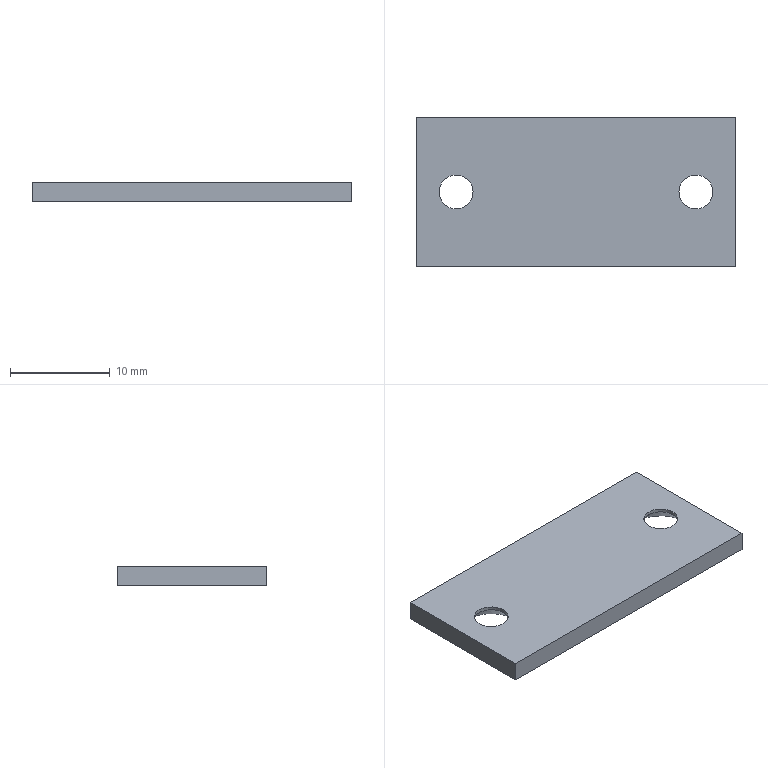Part | SolidWorks | features BaseBody 1 | 1 solid | 14 faces | box 32 x 15 x 2 mm | volume 884.669 mm3 | plane 6 | cone 4 | cylinder 4 | commonest cylinder face diameters 3.4 x4
STEP:
#1=CARTESIAN_POINT('',(-10.3,0.,1.66));
#2=VERTEX_POINT('',#1);
#3=CARTESIAN_POINT('',(-13.7,0.,1.66));
#4=VERTEX_POINT('',#3);
#5=CARTESIAN_POINT('',(-12.,0.,1.66));
#6=DIRECTION('',(0.,0.,-1.));
#7=DIRECTION('',(-1.,0.,0.));
#8=AXIS2_PLACEMENT_3D('',#5,#6,#7);
#9=CIRCLE('',#8,1.7);
#10=EDGE_CURVE('',#2,#4,#9,.T.);
#11=ORIENTED_EDGE('',*,*,#10,.F.);
#12=CARTESIAN_POINT('',(-8.64,0.,0.));
#13=VERTEX_POINT('',#12);
#14=CARTESIAN_POINT('',(-8.64,0.,0.));
#15=DIRECTION('',(0.7071,0.,-0.7071));
#16=VECTOR('',#15,1000.);
#17=LINE('',#14,#16);
#18=EDGE_CURVE('',#2,#13,#17,.T.);
#19=ORIENTED_EDGE('',*,*,#18,.T.);
#20=CARTESIAN_POINT('',(-15.36,0.,0.));
#21=VERTEX_POINT('',#20);
#22=CARTESIAN_POINT('',(-12.,0.,0.));
#23=DIRECTION('',(0.,0.,-1.));
#24=DIRECTION('',(-1.,0.,0.));
#25=AXIS2_PLACEMENT_3D('',#22,#23,#24);
#26=CIRCLE('',#25,3.36);
#27=EDGE_CURVE('',#13,#21,#26,.T.);
#28=ORIENTED_EDGE('',*,*,#27,.T.);
#29=CARTESIAN_POINT('',(-15.36,0.,0.));
#30=DIRECTION('',(-0.7071,0.,-0.7071));
#31=VECTOR('',#30,1000.);
#32=LINE('',#29,#31);
#33=EDGE_CURVE('',#4,#21,#32,.T.);
#34=ORIENTED_EDGE('',*,*,#33,.F.);
#35=EDGE_LOOP('',(#11,#19,#28,#34));
#36=FACE_OUTER_BOUND('',#35,.T.);
#37=CARTESIAN_POINT('',(-12.,0.,0.));
#38=DIRECTION('',(0.,0.,-1.));
#39=DIRECTION('',(-1.,0.,0.));
#40=AXIS2_PLACEMENT_3D('',#37,#38,#39);
#41=CONICAL_SURFACE('',#40,3.36,0.7854);
#42=ADVANCED_FACE('',(#36),#41,.F.);
#43=CARTESIAN_POINT('',(-10.3,0.,2.));
#44=VERTEX_POINT('',#43);
#45=CARTESIAN_POINT('',(-13.7,0.,2.));
#46=VERTEX_POINT('',#45);
#47=CARTESIAN_POINT('',(-12.,0.,2.));
#48=DIRECTION('',(0.,0.,-1.));
#49=DIRECTION('',(-1.,0.,0.));
#50=AXIS2_PLACEMENT_3D('',#47,#48,#49);
#51=CIRCLE('',#50,1.7);
#52=EDGE_CURVE('',#44,#46,#51,.T.);
#53=ORIENTED_EDGE('',*,*,#52,.F.);
#54=CARTESIAN_POINT('',(-10.3,0.,0.));
#55=DIRECTION('',(0.,0.,-1.));
#56=VECTOR('',#55,1000.);
#57=LINE('',#54,#56);
#58=EDGE_CURVE('',#44,#2,#57,.T.);
#59=ORIENTED_EDGE('',*,*,#58,.T.);
#60=ORIENTED_EDGE('',*,*,#10,.T.);
#61=CARTESIAN_POINT('',(-13.7,0.,0.));
#62=DIRECTION('',(0.,0.,-1.));
#63=VECTOR('',#62,1000.);
#64=LINE('',#61,#63);
#65=EDGE_CURVE('',#46,#4,#64,.T.);
#66=ORIENTED_EDGE('',*,*,#65,.F.);
#67=EDGE_LOOP('',(#53,#59,#60,#66));
#68=FACE_OUTER_BOUND('',#67,.T.);
#69=CARTESIAN_POINT('',(-12.,0.,0.));
#70=DIRECTION('',(0.,0.,-1.));
#71=DIRECTION('',(-1.,0.,0.));
#72=AXIS2_PLACEMENT_3D('',#69,#70,#71);
#73=CYLINDRICAL_SURFACE('',#72,1.7);
#74=ADVANCED_FACE('',(#68),#73,.F.);
#75=CARTESIAN_POINT('',(13.7,0.,1.66));
#76=VERTEX_POINT('',#75);
#77=CARTESIAN_POINT('',(10.3,0.,1.66));
#78=VERTEX_POINT('',#77);
#79=CARTESIAN_POINT('',(12.,0.,1.66));
#80=DIRECTION('',(0.,0.,-1.));
#81=DIRECTION('',(-1.,0.,0.));
#82=AXIS2_PLACEMENT_3D('',#79,#80,#81);
#83=CIRCLE('',#82,1.7);
#84=EDGE_CURVE('',#76,#78,#83,.T.);
#85=ORIENTED_EDGE('',*,*,#84,.F.);
#86=CARTESIAN_POINT('',(15.36,0.,0.));
#87=VERTEX_POINT('',#86);
#88=CARTESIAN_POINT('',(15.36,0.,0.));
#89=DIRECTION('',(0.7071,0.,-0.7071));
#90=VECTOR('',#89,1000.);
#91=LINE('',#88,#90);
#92=EDGE_CURVE('',#76,#87,#91,.T.);
#93=ORIENTED_EDGE('',*,*,#92,.T.);
#94=CARTESIAN_POINT('',(8.64,0.,0.));
#95=VERTEX_POINT('',#94);
#96=CARTESIAN_POINT('',(12.,0.,0.));
#97=DIRECTION('',(0.,0.,-1.));
#98=DIRECTION('',(-1.,0.,0.));
#99=AXIS2_PLACEMENT_3D('',#96,#97,#98);
#100=CIRCLE('',#99,3.36);
#101=EDGE_CURVE('',#87,#95,#100,.T.);
#102=ORIENTED_EDGE('',*,*,#101,.T.);
#103=CARTESIAN_POINT('',(8.64,0.,0.));
#104=DIRECTION('',(-0.7071,0.,-0.7071));
#105=VECTOR('',#104,1000.);
#106=LINE('',#103,#105);
#107=EDGE_CURVE('',#78,#95,#106,.T.);
#108=ORIENTED_EDGE('',*,*,#107,.F.);
#109=EDGE_LOOP('',(#85,#93,#102,#108));
#110=FACE_OUTER_BOUND('',#109,.T.);
#111=CARTESIAN_POINT('',(12.,0.,0.));
#112=DIRECTION('',(0.,0.,-1.));
#113=DIRECTION('',(-1.,0.,0.));
#114=AXIS2_PLACEMENT_3D('',#111,#112,#113);
#115=CONICAL_SURFACE('',#114,3.36,0.7854);
#116=ADVANCED_FACE('',(#110),#115,.F.);
#117=CARTESIAN_POINT('',(13.7,0.,2.));
#118=VERTEX_POINT('',#117);
#119=CARTESIAN_POINT('',(10.3,0.,2.));
#120=VERTEX_POINT('',#119);
#121=CARTESIAN_POINT('',(12.,0.,2.));
#122=DIRECTION('',(0.,0.,-1.));
#123=DIRECTION('',(-1.,0.,0.));
#124=AXIS2_PLACEMENT_3D('',#121,#122,#123);
#125=CIRCLE('',#124,1.7);
#126=EDGE_CURVE('',#118,#120,#125,.T.);
#127=ORIENTED_EDGE('',*,*,#126,.F.);
#128=CARTESIAN_POINT('',(13.7,0.,0.));
#129=DIRECTION('',(0.,0.,-1.));
#130=VECTOR('',#129,1000.);
#131=LINE('',#128,#130);
#132=EDGE_CURVE('',#118,#76,#131,.T.);
#133=ORIENTED_EDGE('',*,*,#132,.T.);
#134=ORIENTED_EDGE('',*,*,#84,.T.);
#135=CARTESIAN_POINT('',(10.3,0.,0.));
#136=DIRECTION('',(0.,0.,-1.));
#137=VECTOR('',#136,1000.);
#138=LINE('',#135,#137);
#139=EDGE_CURVE('',#120,#78,#138,.T.);
#140=ORIENTED_EDGE('',*,*,#139,.F.);
#141=EDGE_LOOP('',(#127,#133,#134,#140));
#142=FACE_OUTER_BOUND('',#141,.T.);
#143=CARTESIAN_POINT('',(12.,0.,0.));
#144=DIRECTION('',(0.,0.,-1.));
#145=DIRECTION('',(-1.,0.,0.));
#146=AXIS2_PLACEMENT_3D('',#143,#144,#145);
#147=CYLINDRICAL_SURFACE('',#146,1.7);
#148=ADVANCED_FACE('',(#142),#147,.F.);
#149=CARTESIAN_POINT('',(12.,0.,0.));
#150=DIRECTION('',(0.,0.,-1.));
#151=DIRECTION('',(-1.,0.,0.));
#152=AXIS2_PLACEMENT_3D('',#149,#150,#151);
#153=CIRCLE('',#152,3.36);
#154=EDGE_CURVE('',#95,#87,#153,.T.);
#155=ORIENTED_EDGE('',*,*,#154,.F.);
#156=ORIENTED_EDGE('',*,*,#101,.F.);
#157=EDGE_LOOP('',(#155,#156));
#158=FACE_BOUND('',#157,.T.);
#159=CARTESIAN_POINT('',(-12.,0.,0.));
#160=DIRECTION('',(0.,0.,-1.));
#161=DIRECTION('',(-1.,0.,0.));
#162=AXIS2_PLACEMENT_3D('',#159,#160,#161);
#163=CIRCLE('',#162,3.36);
#164=EDGE_CURVE('',#21,#13,#163,.T.);
#165=ORIENTED_EDGE('',*,*,#164,.F.);
#166=ORIENTED_EDGE('',*,*,#27,.F.);
#167=EDGE_LOOP('',(#165,#166));
#168=FACE_BOUND('',#167,.T.);
#169=CARTESIAN_POINT('',(16.,-7.5,0.));
#170=VERTEX_POINT('',#169);
#171=CARTESIAN_POINT('',(16.,7.5,0.));
#172=VERTEX_POINT('',#171);
#173=CARTESIAN_POINT('',(16.,-7.5,0.));
#174=DIRECTION('',(0.,1.,0.));
#175=VECTOR('',#174,1000.);
#176=LINE('',#173,#175);
#177=EDGE_CURVE('',#170,#172,#176,.T.);
#178=ORIENTED_EDGE('',*,*,#177,.F.);
#179=CARTESIAN_POINT('',(-16.,-7.5,0.));
#180=VERTEX_POINT('',#179);
#181=CARTESIAN_POINT('',(-16.,-7.5,0.));
#182=DIRECTION('',(1.,0.,0.));
#183=VECTOR('',#182,1000.);
#184=LINE('',#181,#183);
#185=EDGE_CURVE('',#180,#170,#184,.T.);
#186=ORIENTED_EDGE('',*,*,#185,.F.);
#187=CARTESIAN_POINT('',(-16.,7.5,0.));
#188=VERTEX_POINT('',#187);
#189=CARTESIAN_POINT('',(-16.,-7.5,0.));
#190=DIRECTION('',(0.,-1.,0.));
#191=VECTOR('',#190,1000.);
#192=LINE('',#189,#191);
#193=EDGE_CURVE('',#188,#180,#192,.T.);
#194=ORIENTED_EDGE('',*,*,#193,.F.);
#195=CARTESIAN_POINT('',(-16.,7.5,0.));
#196=DIRECTION('',(-1.,0.,0.));
#197=VECTOR('',#196,1000.);
#198=LINE('',#195,#197);
#199=EDGE_CURVE('',#172,#188,#198,.T.);
#200=ORIENTED_EDGE('',*,*,#199,.F.);
#201=EDGE_LOOP('',(#178,#186,#194,#200));
#202=FACE_OUTER_BOUND('',#201,.T.);
#203=CARTESIAN_POINT('',(0.,0.,0.));
#204=DIRECTION('',(0.,0.,-1.));
#205=DIRECTION('',(0.,-1.,0.));
#206=AXIS2_PLACEMENT_3D('',#203,#204,#205);
#207=PLANE('',#206);
#208=ADVANCED_FACE('',(#158,#168,#202),#207,.T.);
#209=CARTESIAN_POINT('',(12.,0.,2.));
#210=DIRECTION('',(0.,0.,-1.));
#211=DIRECTION('',(-1.,0.,0.));
#212=AXIS2_PLACEMENT_3D('',#209,#210,#211);
#213=CIRCLE('',#212,1.7);
#214=EDGE_CURVE('',#120,#118,#213,.T.);
#215=ORIENTED_EDGE('',*,*,#214,.T.);
#216=ORIENTED_EDGE('',*,*,#126,.T.);
#217=EDGE_LOOP('',(#215,#216));
#218=FACE_BOUND('',#217,.T.);
#219=CARTESIAN_POINT('',(-12.,0.,2.));
#220=DIRECTION('',(0.,0.,-1.));
#221=DIRECTION('',(-1.,0.,0.));
#222=AXIS2_PLACEMENT_3D('',#219,#220,#221);
#223=CIRCLE('',#222,1.7);
#224=EDGE_CURVE('',#46,#44,#223,.T.);
#225=ORIENTED_EDGE('',*,*,#224,.T.);
#226=ORIENTED_EDGE('',*,*,#52,.T.);
#227=EDGE_LOOP('',(#225,#226));
#228=FACE_BOUND('',#227,.T.);
#229=CARTESIAN_POINT('',(16.,-7.5,2.));
#230=VERTEX_POINT('',#229);
#231=CARTESIAN_POINT('',(16.,7.5,2.));
#232=VERTEX_POINT('',#231);
#233=CARTESIAN_POINT('',(16.,-7.5,2.));
#234=DIRECTION('',(0.,1.,0.));
#235=VECTOR('',#234,1000.);
#236=LINE('',#233,#235);
#237=EDGE_CURVE('',#230,#232,#236,.T.);
#238=ORIENTED_EDGE('',*,*,#237,.T.);
#239=CARTESIAN_POINT('',(-16.,7.5,2.));
#240=VERTEX_POINT('',#239);
#241=CARTESIAN_POINT('',(-16.,7.5,2.));
#242=DIRECTION('',(-1.,0.,0.));
#243=VECTOR('',#242,1000.);
#244=LINE('',#241,#243);
#245=EDGE_CURVE('',#232,#240,#244,.T.);
#246=ORIENTED_EDGE('',*,*,#245,.T.);
#247=CARTESIAN_POINT('',(-16.,-7.5,2.));
#248=VERTEX_POINT('',#247);
#249=CARTESIAN_POINT('',(-16.,-7.5,2.));
#250=DIRECTION('',(0.,-1.,0.));
#251=VECTOR('',#250,1000.);
#252=LINE('',#249,#251);
#253=EDGE_CURVE('',#240,#248,#252,.T.);
#254=ORIENTED_EDGE('',*,*,#253,.T.);
#255=CARTESIAN_POINT('',(-16.,-7.5,2.));
#256=DIRECTION('',(1.,0.,0.));
#257=VECTOR('',#256,1000.);
#258=LINE('',#255,#257);
#259=EDGE_CURVE('',#248,#230,#258,.T.);
#260=ORIENTED_EDGE('',*,*,#259,.T.);
#261=EDGE_LOOP('',(#238,#246,#254,#260));
#262=FACE_OUTER_BOUND('',#261,.T.);
#263=CARTESIAN_POINT('',(0.,0.,2.));
#264=DIRECTION('',(0.,0.,-1.));
#265=DIRECTION('',(0.,-1.,0.));
#266=AXIS2_PLACEMENT_3D('',#263,#264,#265);
#267=PLANE('',#266);
#268=ADVANCED_FACE('',(#218,#228,#262),#267,.F.);
#269=ORIENTED_EDGE('',*,*,#185,.T.);
#270=CARTESIAN_POINT('',(16.,-7.5,2.));
#271=DIRECTION('',(0.,0.,-1.));
#272=VECTOR('',#271,1000.);
#273=LINE('',#270,#272);
#274=EDGE_CURVE('',#230,#170,#273,.T.);
#275=ORIENTED_EDGE('',*,*,#274,.F.);
#276=ORIENTED_EDGE('',*,*,#259,.F.);
#277=CARTESIAN_POINT('',(-16.,-7.5,2.));
#278=DIRECTION('',(0.,0.,-1.));
#279=VECTOR('',#278,1000.);
#280=LINE('',#277,#279);
#281=EDGE_CURVE('',#248,#180,#280,.T.);
#282=ORIENTED_EDGE('',*,*,#281,.T.);
#283=EDGE_LOOP('',(#269,#275,#276,#282));
#284=FACE_OUTER_BOUND('',#283,.T.);
#285=CARTESIAN_POINT('',(-16.,-7.5,2.));
#286=DIRECTION('',(0.,1.,0.));
#287=DIRECTION('',(1.,0.,0.));
#288=AXIS2_PLACEMENT_3D('',#285,#286,#287);
#289=PLANE('',#288);
#290=ADVANCED_FACE('',(#284),#289,.F.);
#291=ORIENTED_EDGE('',*,*,#193,.T.);
#292=ORIENTED_EDGE('',*,*,#281,.F.);
#293=ORIENTED_EDGE('',*,*,#253,.F.);
#294=CARTESIAN_POINT('',(-16.,7.5,2.));
#295=DIRECTION('',(0.,0.,-1.));
#296=VECTOR('',#295,1000.);
#297=LINE('',#294,#296);
#298=EDGE_CURVE('',#240,#188,#297,.T.);
#299=ORIENTED_EDGE('',*,*,#298,.T.);
#300=EDGE_LOOP('',(#291,#292,#293,#299));
#301=FACE_OUTER_BOUND('',#300,.T.);
#302=CARTESIAN_POINT('',(-16.,-7.5,2.));
#303=DIRECTION('',(1.,0.,0.));
#304=DIRECTION('',(0.,1.,0.));
#305=AXIS2_PLACEMENT_3D('',#302,#303,#304);
#306=PLANE('',#305);
#307=ADVANCED_FACE('',(#301),#306,.F.);
#308=ORIENTED_EDGE('',*,*,#199,.T.);
#309=ORIENTED_EDGE('',*,*,#298,.F.);
#310=ORIENTED_EDGE('',*,*,#245,.F.);
#311=CARTESIAN_POINT('',(16.,7.5,2.));
#312=DIRECTION('',(0.,0.,-1.));
#313=VECTOR('',#312,1000.);
#314=LINE('',#311,#313);
#315=EDGE_CURVE('',#232,#172,#314,.T.);
#316=ORIENTED_EDGE('',*,*,#315,.T.);
#317=EDGE_LOOP('',(#308,#309,#310,#316));
#318=FACE_OUTER_BOUND('',#317,.T.);
#319=CARTESIAN_POINT('',(-16.,7.5,2.));
#320=DIRECTION('',(0.,-1.,0.));
#321=DIRECTION('',(0.,0.,-1.));
#322=AXIS2_PLACEMENT_3D('',#319,#320,#321);
#323=PLANE('',#322);
#324=ADVANCED_FACE('',(#318),#323,.F.);
#325=ORIENTED_EDGE('',*,*,#177,.T.);
#326=ORIENTED_EDGE('',*,*,#315,.F.);
#327=ORIENTED_EDGE('',*,*,#237,.F.);
#328=ORIENTED_EDGE('',*,*,#274,.T.);
#329=EDGE_LOOP('',(#325,#326,#327,#328));
#330=FACE_OUTER_BOUND('',#329,.T.);
#331=CARTESIAN_POINT('',(16.,-7.5,2.));
#332=DIRECTION('',(-1.,0.,0.));
#333=DIRECTION('',(0.,0.,1.));
#334=AXIS2_PLACEMENT_3D('',#331,#332,#333);
#335=PLANE('',#334);
#336=ADVANCED_FACE('',(#330),#335,.F.);
#337=ORIENTED_EDGE('',*,*,#132,.F.);
#338=ORIENTED_EDGE('',*,*,#214,.F.);
#339=ORIENTED_EDGE('',*,*,#139,.T.);
#340=CARTESIAN_POINT('',(12.,0.,1.66));
#341=DIRECTION('',(0.,0.,-1.));
#342=DIRECTION('',(-1.,0.,0.));
#343=AXIS2_PLACEMENT_3D('',#340,#341,#342);
#344=CIRCLE('',#343,1.7);
#345=EDGE_CURVE('',#78,#76,#344,.T.);
#346=ORIENTED_EDGE('',*,*,#345,.T.);
#347=EDGE_LOOP('',(#337,#338,#339,#346));
#348=FACE_OUTER_BOUND('',#347,.T.);
#349=CARTESIAN_POINT('',(12.,0.,0.));
#350=DIRECTION('',(0.,0.,-1.));
#351=DIRECTION('',(-1.,0.,0.));
#352=AXIS2_PLACEMENT_3D('',#349,#350,#351);
#353=CYLINDRICAL_SURFACE('',#352,1.7);
#354=ADVANCED_FACE('',(#348),#353,.F.);
#355=ORIENTED_EDGE('',*,*,#92,.F.);
#356=ORIENTED_EDGE('',*,*,#345,.F.);
#357=ORIENTED_EDGE('',*,*,#107,.T.);
#358=ORIENTED_EDGE('',*,*,#154,.T.);
#359=EDGE_LOOP('',(#355,#356,#357,#358));
#360=FACE_OUTER_BOUND('',#359,.T.);
#361=CARTESIAN_POINT('',(12.,0.,0.));
#362=DIRECTION('',(0.,0.,-1.));
#363=DIRECTION('',(-1.,0.,0.));
#364=AXIS2_PLACEMENT_3D('',#361,#362,#363);
#365=CONICAL_SURFACE('',#364,3.36,0.7854);
#366=ADVANCED_FACE('',(#360),#365,.F.);
#367=ORIENTED_EDGE('',*,*,#58,.F.);
#368=ORIENTED_EDGE('',*,*,#224,.F.);
#369=ORIENTED_EDGE('',*,*,#65,.T.);
#370=CARTESIAN_POINT('',(-12.,0.,1.66));
#371=DIRECTION('',(0.,0.,-1.));
#372=DIRECTION('',(-1.,0.,0.));
#373=AXIS2_PLACEMENT_3D('',#370,#371,#372);
#374=CIRCLE('',#373,1.7);
#375=EDGE_CURVE('',#4,#2,#374,.T.);
#376=ORIENTED_EDGE('',*,*,#375,.T.);
#377=EDGE_LOOP('',(#367,#368,#369,#376));
#378=FACE_OUTER_BOUND('',#377,.T.);
#379=CARTESIAN_POINT('',(-12.,0.,0.));
#380=DIRECTION('',(0.,0.,-1.));
#381=DIRECTION('',(-1.,0.,0.));
#382=AXIS2_PLACEMENT_3D('',#379,#380,#381);
#383=CYLINDRICAL_SURFACE('',#382,1.7);
#384=ADVANCED_FACE('',(#378),#383,.F.);
#385=ORIENTED_EDGE('',*,*,#18,.F.);
#386=ORIENTED_EDGE('',*,*,#375,.F.);
#387=ORIENTED_EDGE('',*,*,#33,.T.);
#388=ORIENTED_EDGE('',*,*,#164,.T.);
#389=EDGE_LOOP('',(#385,#386,#387,#388));
#390=FACE_OUTER_BOUND('',#389,.T.);
#391=CARTESIAN_POINT('',(-12.,0.,0.));
#392=DIRECTION('',(0.,0.,-1.));
#393=DIRECTION('',(-1.,0.,0.));
#394=AXIS2_PLACEMENT_3D('',#391,#392,#393);
#395=CONICAL_SURFACE('',#394,3.36,0.7854);
#396=ADVANCED_FACE('',(#390),#395,.F.);
#397=CLOSED_SHELL('',(#42,#74,#116,#148,#208,#268,#290,#307,#324,#336,#354,#366,#384,#396));
#398=MANIFOLD_SOLID_BREP('',#397);
#399=CARTESIAN_POINT('',(0.,0.,0.));
#400=DIRECTION('',(0.,0.,1.));
#401=DIRECTION('',(1.,0.,0.));
#402=AXIS2_PLACEMENT_3D('',#399,#400,#401);
#403=(LENGTH_UNIT()NAMED_UNIT(*)SI_UNIT(.MILLI.,.METRE.));
#404=UNCERTAINTY_MEASURE_WITH_UNIT(LENGTH_MEASURE(0.00001),#403,'','');
#405=(NAMED_UNIT(*)PLANE_ANGLE_UNIT()SI_UNIT($,.RADIAN.));
#406=(NAMED_UNIT(*)SI_UNIT($,.STERADIAN.)SOLID_ANGLE_UNIT());
#407=(GEOMETRIC_REPRESENTATION_CONTEXT(3)GLOBAL_UNCERTAINTY_ASSIGNED_CONTEXT((#404))GLOBAL_UNIT_ASSIGNED_CONTEXT((#403,#405,#406))REPRESENTATION_CONTEXT('',''));
#408=ADVANCED_BREP_SHAPE_REPRESENTATION('',(#398,#402),#407);